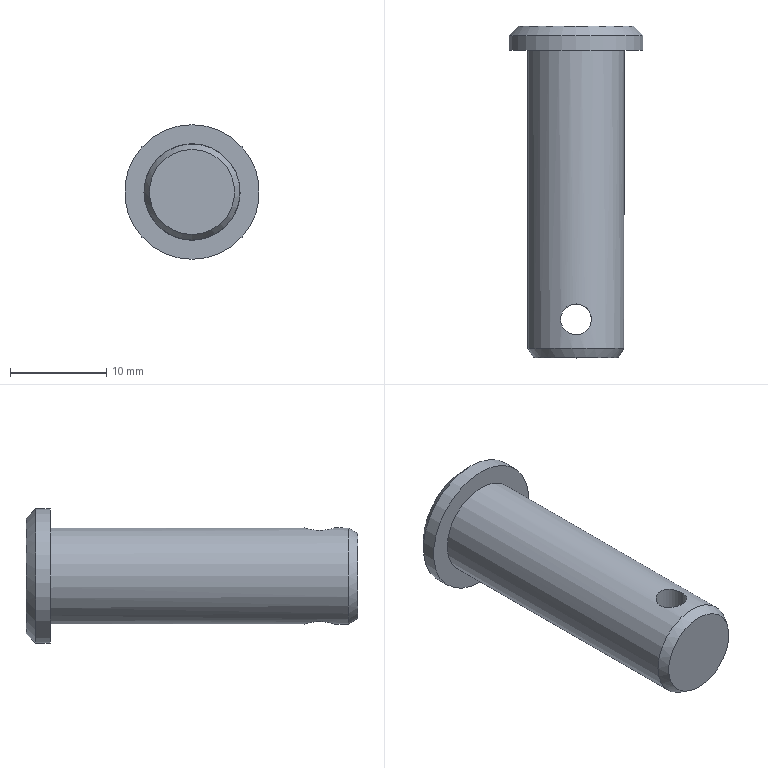Part | NX | features solid 2 | 1 solid | 8 faces | box 14 x 34.5 x 14 mm | volume 2789 mm3 | cylinder 3 | plane 3 | cone 2 | commonest cylinder face diameters 3.2 x1 10 x1 14 x1
STEP:
#1=CARTESIAN_POINT('',(-910.,67.4,-129.));
#2=VERTEX_POINT('',#1);
#3=CARTESIAN_POINT('',(-908.746,67.747,-128.872));
#4=CARTESIAN_POINT('',(-910.,67.226,-129.064));
#5=CARTESIAN_POINT('',(-911.254,67.747,-128.872));
#6=CARTESIAN_POINT('',(-911.773,68.998,-128.67));
#7=CARTESIAN_POINT('',(-911.253,70.254,-128.872));
#8=CARTESIAN_POINT('',(-910.001,70.773,-129.064));
#9=CARTESIAN_POINT('',(-908.746,70.254,-128.872));
#10=CARTESIAN_POINT('',(-908.227,69.,-128.67));
#11=CARTESIAN_POINT('',(-908.746,67.747,-128.872));
#12=CARTESIAN_POINT('',(-910.,67.226,-129.064));
#13=CARTESIAN_POINT('',(-911.254,67.747,-128.872));
#14=B_SPLINE_CURVE_WITH_KNOTS('',3,(#3,#4,#5,#6,#7,#8,#9,#10,#11,#12,#13),.UNSPECIFIED.,.T.,.F.,(1,1,1,1,1,1,1,1,1,1,1,1,1,1,1),(-0.003776,-0.002518,-0.001259,0.,0.001259,0.002518,0.003776,0.005035,0.006294,0.007553,0.008811,0.01007,0.01133,0.01259,0.01385),.UNSPECIFIED.);
#15=EDGE_CURVE('',#2,#2,#14,.T.);
#16=ORIENTED_EDGE('',*,*,#15,.F.);
#17=EDGE_LOOP('',(#16));
#18=FACE_BOUND('',#17,.T.);
#19=CARTESIAN_POINT('',(-910.,66.,-129.));
#20=VERTEX_POINT('',#19);
#21=CARTESIAN_POINT('',(-910.,66.,-124.));
#22=DIRECTION('',(0.,1.,0.));
#23=DIRECTION('',(0.,0.,-1.));
#24=AXIS2_PLACEMENT_3D('',#21,#22,#23);
#25=CIRCLE('',#24,5.);
#26=EDGE_CURVE('',#20,#20,#25,.T.);
#27=ORIENTED_EDGE('',*,*,#26,.T.);
#28=EDGE_LOOP('',(#27));
#29=FACE_BOUND('',#28,.T.);
#30=CARTESIAN_POINT('',(-915.,97.,-124.));
#31=VERTEX_POINT('',#30);
#32=CARTESIAN_POINT('',(-910.,97.,-124.));
#33=DIRECTION('',(0.,1.,0.));
#34=DIRECTION('',(-1.,0.,0.));
#35=AXIS2_PLACEMENT_3D('',#32,#33,#34);
#36=CIRCLE('',#35,5.);
#37=EDGE_CURVE('',#31,#31,#36,.T.);
#38=ORIENTED_EDGE('',*,*,#37,.F.);
#39=EDGE_LOOP('',(#38));
#40=FACE_BOUND('',#39,.T.);
#41=CARTESIAN_POINT('',(-910.,70.6,-119.));
#42=VERTEX_POINT('',#41);
#43=CARTESIAN_POINT('',(-908.746,70.253,-119.128));
#44=CARTESIAN_POINT('',(-910.,70.774,-118.936));
#45=CARTESIAN_POINT('',(-911.254,70.253,-119.128));
#46=CARTESIAN_POINT('',(-911.773,69.002,-119.33));
#47=CARTESIAN_POINT('',(-911.253,67.746,-119.128));
#48=CARTESIAN_POINT('',(-910.001,67.227,-118.936));
#49=CARTESIAN_POINT('',(-908.746,67.746,-119.128));
#50=CARTESIAN_POINT('',(-908.227,69.,-119.33));
#51=CARTESIAN_POINT('',(-908.746,70.253,-119.128));
#52=CARTESIAN_POINT('',(-910.,70.774,-118.936));
#53=CARTESIAN_POINT('',(-911.254,70.253,-119.128));
#54=B_SPLINE_CURVE_WITH_KNOTS('',3,(#43,#44,#45,#46,#47,#48,#49,#50,#51,#52,#53),.UNSPECIFIED.,.T.,.F.,(1,1,1,1,1,1,1,1,1,1,1,1,1,1,1),(-0.003776,-0.002518,-0.001259,0.,0.001259,0.002518,0.003776,0.005035,0.006294,0.007553,0.008811,0.01007,0.01133,0.01259,0.01385),.UNSPECIFIED.);
#55=EDGE_CURVE('',#42,#42,#54,.T.);
#56=ORIENTED_EDGE('',*,*,#55,.F.);
#57=EDGE_LOOP('',(#56));
#58=FACE_BOUND('',#57,.T.);
#59=CARTESIAN_POINT('',(-910.,99.5,-124.));
#60=DIRECTION('',(0.,-1.,0.));
#61=DIRECTION('',(0.,0.,1.));
#62=AXIS2_PLACEMENT_3D('',#59,#60,#61);
#63=CYLINDRICAL_SURFACE('',#62,5.);
#64=ADVANCED_FACE('',(#18,#29,#40,#58),#63,.T.);
#65=CARTESIAN_POINT('',(-910.,65.,-128.423));
#66=VERTEX_POINT('',#65);
#67=CARTESIAN_POINT('',(-910.,65.,-124.));
#68=DIRECTION('',(0.,1.,0.));
#69=DIRECTION('',(0.,0.,-1.));
#70=AXIS2_PLACEMENT_3D('',#67,#68,#69);
#71=CIRCLE('',#70,4.423);
#72=EDGE_CURVE('',#66,#66,#71,.F.);
#73=ORIENTED_EDGE('',*,*,#72,.T.);
#74=EDGE_LOOP('',(#73));
#75=FACE_BOUND('',#74,.T.);
#76=CARTESIAN_POINT('',(-910.,65.,-124.));
#77=DIRECTION('',(0.,1.,0.));
#78=DIRECTION('',(0.,0.,-1.));
#79=AXIS2_PLACEMENT_3D('',#76,#77,#78);
#80=PLANE('',#79);
#81=ADVANCED_FACE('',(#75),#80,.F.);
#82=CARTESIAN_POINT('',(-910.,98.5,-131.));
#83=VERTEX_POINT('',#82);
#84=CARTESIAN_POINT('',(-910.,98.5,-124.));
#85=DIRECTION('',(0.,1.,0.));
#86=DIRECTION('',(0.,0.,-1.));
#87=AXIS2_PLACEMENT_3D('',#84,#85,#86);
#88=CIRCLE('',#87,7.);
#89=EDGE_CURVE('',#83,#83,#88,.F.);
#90=ORIENTED_EDGE('',*,*,#89,.T.);
#91=EDGE_LOOP('',(#90));
#92=FACE_BOUND('',#91,.T.);
#93=CARTESIAN_POINT('',(-910.,97.,-117.));
#94=VERTEX_POINT('',#93);
#95=CARTESIAN_POINT('',(-910.,97.,-124.));
#96=DIRECTION('',(0.,-1.,0.));
#97=DIRECTION('',(0.,0.,1.));
#98=AXIS2_PLACEMENT_3D('',#95,#96,#97);
#99=CIRCLE('',#98,7.);
#100=EDGE_CURVE('',#94,#94,#99,.F.);
#101=ORIENTED_EDGE('',*,*,#100,.T.);
#102=EDGE_LOOP('',(#101));
#103=FACE_BOUND('',#102,.T.);
#104=CARTESIAN_POINT('',(-910.,99.5,-124.));
#105=DIRECTION('',(0.,-1.,0.));
#106=DIRECTION('',(0.,0.,1.));
#107=AXIS2_PLACEMENT_3D('',#104,#105,#106);
#108=CYLINDRICAL_SURFACE('',#107,7.);
#109=ADVANCED_FACE('',(#92,#103),#108,.T.);
#110=ORIENTED_EDGE('',*,*,#100,.F.);
#111=EDGE_LOOP('',(#110));
#112=FACE_BOUND('',#111,.T.);
#113=ORIENTED_EDGE('',*,*,#37,.T.);
#114=EDGE_LOOP('',(#113));
#115=FACE_BOUND('',#114,.T.);
#116=CARTESIAN_POINT('',(-910.,97.,-124.));
#117=DIRECTION('',(0.,-1.,0.));
#118=DIRECTION('',(0.,0.,1.));
#119=AXIS2_PLACEMENT_3D('',#116,#117,#118);
#120=PLANE('',#119);
#121=ADVANCED_FACE('',(#112,#115),#120,.T.);
#122=CARTESIAN_POINT('',(-910.,99.5,-130.));
#123=VERTEX_POINT('',#122);
#124=CARTESIAN_POINT('',(-910.,99.5,-124.));
#125=DIRECTION('',(0.,1.,0.));
#126=DIRECTION('',(0.,0.,-1.));
#127=AXIS2_PLACEMENT_3D('',#124,#125,#126);
#128=CIRCLE('',#127,6.);
#129=EDGE_CURVE('',#123,#123,#128,.T.);
#130=ORIENTED_EDGE('',*,*,#129,.T.);
#131=EDGE_LOOP('',(#130));
#132=FACE_BOUND('',#131,.T.);
#133=CARTESIAN_POINT('',(-910.,99.5,-124.));
#134=DIRECTION('',(0.,1.,0.));
#135=DIRECTION('',(0.,0.,-1.));
#136=AXIS2_PLACEMENT_3D('',#133,#134,#135);
#137=PLANE('',#136);
#138=ADVANCED_FACE('',(#132),#137,.T.);
#139=ORIENTED_EDGE('',*,*,#89,.F.);
#140=EDGE_LOOP('',(#139));
#141=FACE_BOUND('',#140,.T.);
#142=ORIENTED_EDGE('',*,*,#129,.F.);
#143=EDGE_LOOP('',(#142));
#144=FACE_BOUND('',#143,.T.);
#145=CARTESIAN_POINT('',(-910.,99.5,-124.));
#146=DIRECTION('',(0.,-1.,0.));
#147=DIRECTION('',(0.,0.,1.));
#148=AXIS2_PLACEMENT_3D('',#145,#146,#147);
#149=CONICAL_SURFACE('',#148,6.,0.7854);
#150=ADVANCED_FACE('',(#141,#144),#149,.T.);
#151=ORIENTED_EDGE('',*,*,#72,.F.);
#152=EDGE_LOOP('',(#151));
#153=FACE_BOUND('',#152,.T.);
#154=ORIENTED_EDGE('',*,*,#26,.F.);
#155=EDGE_LOOP('',(#154));
#156=FACE_BOUND('',#155,.T.);
#157=CARTESIAN_POINT('',(-910.,66.,-124.));
#158=DIRECTION('',(0.,1.,0.));
#159=DIRECTION('',(0.,0.,-1.));
#160=AXIS2_PLACEMENT_3D('',#157,#158,#159);
#161=CONICAL_SURFACE('',#160,5.,0.5236);
#162=ADVANCED_FACE('',(#153,#156),#161,.T.);
#163=ORIENTED_EDGE('',*,*,#15,.T.);
#164=EDGE_LOOP('',(#163));
#165=FACE_BOUND('',#164,.T.);
#166=ORIENTED_EDGE('',*,*,#55,.T.);
#167=EDGE_LOOP('',(#166));
#168=FACE_BOUND('',#167,.T.);
#169=CARTESIAN_POINT('',(-910.,69.,-34.));
#170=DIRECTION('',(0.,0.,-1.));
#171=DIRECTION('',(0.,-1.,0.));
#172=AXIS2_PLACEMENT_3D('',#169,#170,#171);
#173=CYLINDRICAL_SURFACE('',#172,1.6);
#174=ADVANCED_FACE('',(#165,#168),#173,.F.);
#175=CLOSED_SHELL('',(#64,#81,#109,#121,#138,#150,#162,#174));
#176=MANIFOLD_SOLID_BREP('',#175);
#177=(LENGTH_UNIT()NAMED_UNIT(*)SI_UNIT(.MILLI.,.METRE.));
#178=UNCERTAINTY_MEASURE_WITH_UNIT(LENGTH_MEASURE(0.0508),#177,'','');
#179=(NAMED_UNIT(*)PLANE_ANGLE_UNIT()SI_UNIT($,.RADIAN.));
#180=(NAMED_UNIT(*)SI_UNIT($,.STERADIAN.)SOLID_ANGLE_UNIT());
#181=(GEOMETRIC_REPRESENTATION_CONTEXT(3)GLOBAL_UNCERTAINTY_ASSIGNED_CONTEXT((#178))GLOBAL_UNIT_ASSIGNED_CONTEXT((#177,#179,#180))REPRESENTATION_CONTEXT('',''));
#182=ADVANCED_BREP_SHAPE_REPRESENTATION('',(#176),#181);